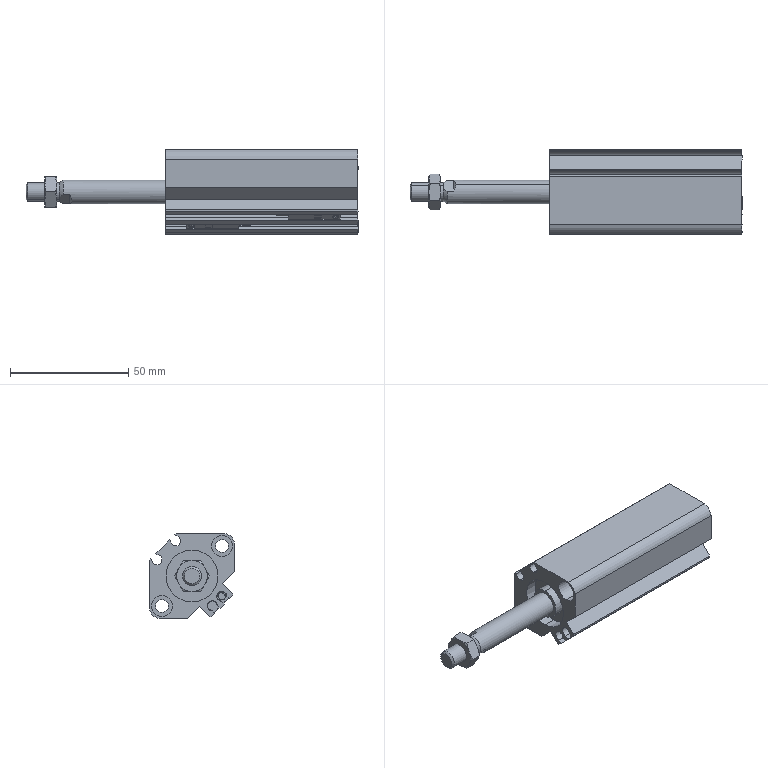Part | SolidWorks | features AEMSimFeature 1 | 5 solids | 188 faces | box 140.657 x 36 x 36 mm | volume 68921 mm3 | plane 90 | cylinder 74 | cone 24 | commonest cylinder face diameters 4.26 x10 0.6 x8 9 x8 2.7 x6 4 x6 10 x6